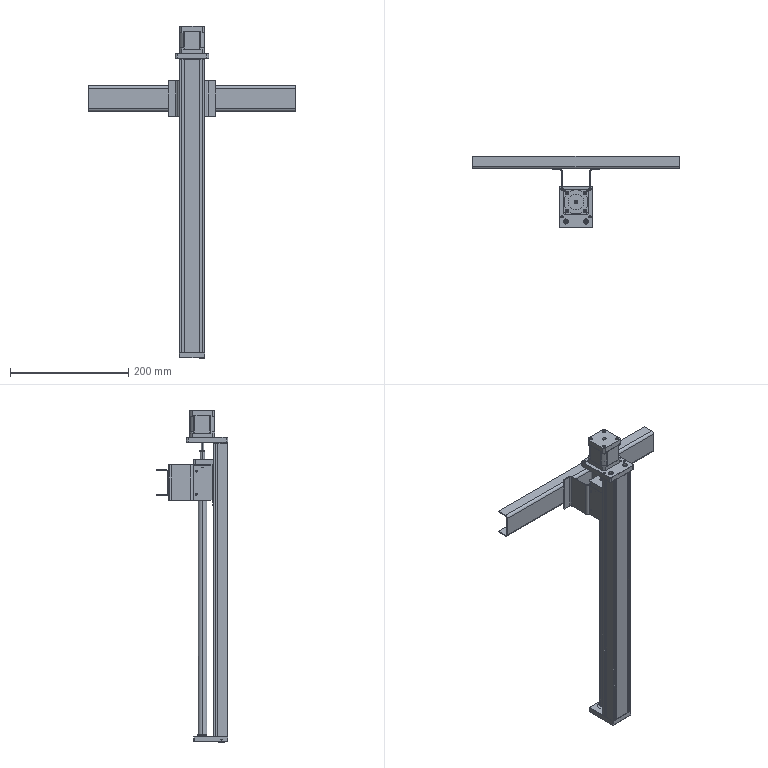Part | SolidWorks | 19 solids | 2043 faces | box 350 x 121.3 x 561.8 mm | volume 585009 mm3 | cone 1336 | plane 402 | cylinder 281 | spline 16 | torus 8 | commonest cylinder face diameters 3.3 x48 8 x27 6.5 x24 3 x16 3.4 x16 6 x16